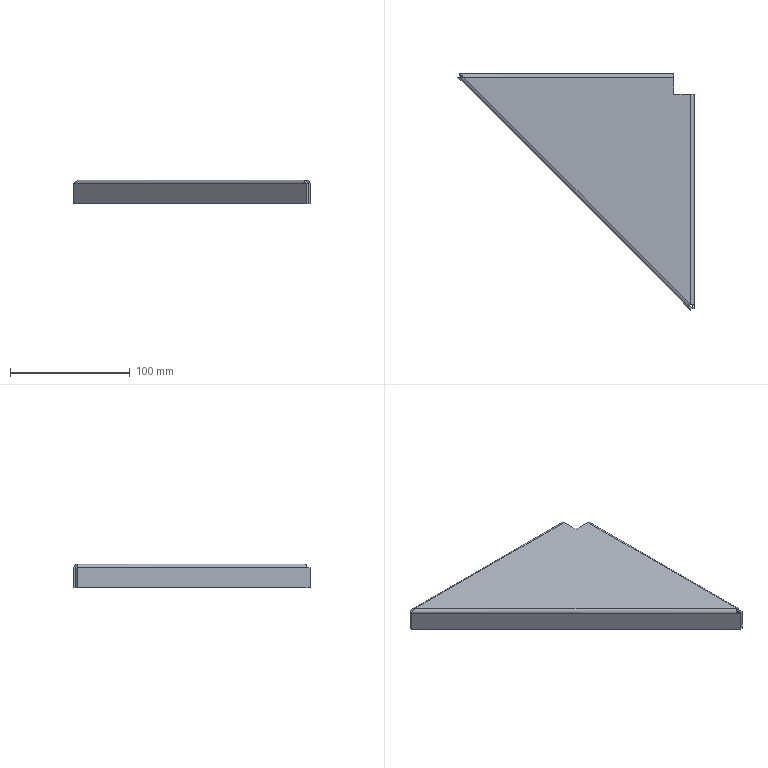Part | NX | features solid 2 | 1 solid | 45 faces | box 197.436 x 197.436 x 20 mm | volume 45854 mm3 | cylinder 22 | plane 21 | spline 2 | commonest cylinder face diameters 6 x19 3 x3
STEP:
#1=CARTESIAN_POINT('',(1090.,488.,1292.));
#2=VERTEX_POINT('',#1);
#3=CARTESIAN_POINT('',(1090.,488.,1275.));
#4=VERTEX_POINT('',#3);
#5=CARTESIAN_POINT('',(1090.,488.,1295.));
#6=DIRECTION('',(0.,0.,-1.));
#7=VECTOR('',#6,1000.);
#8=LINE('',#5,#7);
#9=EDGE_CURVE('',#2,#4,#8,.T.);
#10=ORIENTED_EDGE('',*,*,#9,.T.);
#11=CARTESIAN_POINT('',(1088.5,488.,1275.));
#12=VERTEX_POINT('',#11);
#13=CARTESIAN_POINT('',(1090.,488.,1275.));
#14=DIRECTION('',(1.,0.,0.));
#15=VECTOR('',#14,1000.);
#16=LINE('',#13,#15);
#17=EDGE_CURVE('',#12,#4,#16,.T.);
#18=ORIENTED_EDGE('',*,*,#17,.F.);
#19=CARTESIAN_POINT('',(1088.5,488.,1292.));
#20=VERTEX_POINT('',#19);
#21=CARTESIAN_POINT('',(1088.5,488.,1295.));
#22=DIRECTION('',(0.,0.,-1.));
#23=VECTOR('',#22,1000.);
#24=LINE('',#21,#23);
#25=EDGE_CURVE('',#20,#12,#24,.T.);
#26=ORIENTED_EDGE('',*,*,#25,.F.);
#27=CARTESIAN_POINT('',(1087.,488.,1293.5));
#28=VERTEX_POINT('',#27);
#29=CARTESIAN_POINT('',(1087.,488.,1292.));
#30=DIRECTION('',(0.,1.,0.));
#31=DIRECTION('',(0.,0.,1.));
#32=AXIS2_PLACEMENT_3D('',#29,#30,#31);
#33=CIRCLE('',#32,1.5);
#34=EDGE_CURVE('',#28,#20,#33,.T.);
#35=ORIENTED_EDGE('',*,*,#34,.F.);
#36=CARTESIAN_POINT('',(1073.,488.,1293.5));
#37=VERTEX_POINT('',#36);
#38=CARTESIAN_POINT('',(990.,488.,1293.5));
#39=DIRECTION('',(1.,0.,0.));
#40=VECTOR('',#39,1000.);
#41=LINE('',#38,#40);
#42=EDGE_CURVE('',#37,#28,#41,.T.);
#43=ORIENTED_EDGE('',*,*,#42,.F.);
#44=CARTESIAN_POINT('',(1073.,488.,1295.));
#45=VERTEX_POINT('',#44);
#46=CARTESIAN_POINT('',(1073.,488.,1295.));
#47=DIRECTION('',(0.,0.,1.));
#48=VECTOR('',#47,1000.);
#49=LINE('',#46,#48);
#50=EDGE_CURVE('',#37,#45,#49,.T.);
#51=ORIENTED_EDGE('',*,*,#50,.T.);
#52=CARTESIAN_POINT('',(1087.,488.,1295.));
#53=VERTEX_POINT('',#52);
#54=CARTESIAN_POINT('',(990.,488.,1295.));
#55=DIRECTION('',(1.,0.,0.));
#56=VECTOR('',#55,1000.);
#57=LINE('',#54,#56);
#58=EDGE_CURVE('',#45,#53,#57,.T.);
#59=ORIENTED_EDGE('',*,*,#58,.T.);
#60=CARTESIAN_POINT('',(1087.,488.,1292.));
#61=DIRECTION('',(0.,1.,0.));
#62=DIRECTION('',(0.,0.,1.));
#63=AXIS2_PLACEMENT_3D('',#60,#61,#62);
#64=CIRCLE('',#63,3.);
#65=EDGE_CURVE('',#53,#2,#64,.T.);
#66=ORIENTED_EDGE('',*,*,#65,.T.);
#67=EDGE_LOOP('',(#10,#18,#26,#35,#43,#51,#59,#66));
#68=FACE_BOUND('',#67,.T.);
#69=CARTESIAN_POINT('',(1090.,488.,1295.));
#70=DIRECTION('',(0.,-1.,0.));
#71=DIRECTION('',(-1.,0.,0.));
#72=AXIS2_PLACEMENT_3D('',#69,#70,#71);
#73=PLANE('',#72);
#74=ADVANCED_FACE('',(#68),#73,.F.);
#75=CARTESIAN_POINT('',(1073.,502.,1295.));
#76=VERTEX_POINT('',#75);
#77=CARTESIAN_POINT('',(1073.,405.,1295.));
#78=DIRECTION('',(0.,-1.,0.));
#79=VECTOR('',#78,1000.);
#80=LINE('',#77,#79);
#81=EDGE_CURVE('',#76,#45,#80,.T.);
#82=ORIENTED_EDGE('',*,*,#81,.T.);
#83=ORIENTED_EDGE('',*,*,#50,.F.);
#84=CARTESIAN_POINT('',(1073.,502.,1293.5));
#85=VERTEX_POINT('',#84);
#86=CARTESIAN_POINT('',(1073.,405.,1293.5));
#87=DIRECTION('',(0.,-1.,0.));
#88=VECTOR('',#87,1000.);
#89=LINE('',#86,#88);
#90=EDGE_CURVE('',#85,#37,#89,.T.);
#91=ORIENTED_EDGE('',*,*,#90,.F.);
#92=CARTESIAN_POINT('',(1073.,503.5,1292.));
#93=VERTEX_POINT('',#92);
#94=CARTESIAN_POINT('',(1073.,502.,1292.));
#95=DIRECTION('',(1.,0.,0.));
#96=DIRECTION('',(0.,1.,0.));
#97=AXIS2_PLACEMENT_3D('',#94,#95,#96);
#98=CIRCLE('',#97,1.5);
#99=EDGE_CURVE('',#93,#85,#98,.T.);
#100=ORIENTED_EDGE('',*,*,#99,.F.);
#101=CARTESIAN_POINT('',(1073.,503.5,1275.));
#102=VERTEX_POINT('',#101);
#103=CARTESIAN_POINT('',(1073.,503.5,1295.));
#104=DIRECTION('',(0.,0.,1.));
#105=VECTOR('',#104,1000.);
#106=LINE('',#103,#105);
#107=EDGE_CURVE('',#102,#93,#106,.T.);
#108=ORIENTED_EDGE('',*,*,#107,.F.);
#109=CARTESIAN_POINT('',(1073.,505.,1275.));
#110=VERTEX_POINT('',#109);
#111=CARTESIAN_POINT('',(1073.,505.,1275.));
#112=DIRECTION('',(0.,1.,0.));
#113=VECTOR('',#112,1000.);
#114=LINE('',#111,#113);
#115=EDGE_CURVE('',#102,#110,#114,.T.);
#116=ORIENTED_EDGE('',*,*,#115,.T.);
#117=CARTESIAN_POINT('',(1073.,505.,1292.));
#118=VERTEX_POINT('',#117);
#119=CARTESIAN_POINT('',(1073.,505.,1295.));
#120=DIRECTION('',(0.,0.,1.));
#121=VECTOR('',#120,1000.);
#122=LINE('',#119,#121);
#123=EDGE_CURVE('',#110,#118,#122,.T.);
#124=ORIENTED_EDGE('',*,*,#123,.T.);
#125=CARTESIAN_POINT('',(1073.,502.,1292.));
#126=DIRECTION('',(1.,0.,0.));
#127=DIRECTION('',(0.,0.,-1.));
#128=AXIS2_PLACEMENT_3D('',#125,#126,#127);
#129=CIRCLE('',#128,3.);
#130=EDGE_CURVE('',#118,#76,#129,.T.);
#131=ORIENTED_EDGE('',*,*,#130,.T.);
#132=EDGE_LOOP('',(#82,#83,#91,#100,#108,#116,#124,#131));
#133=FACE_BOUND('',#132,.T.);
#134=CARTESIAN_POINT('',(1073.,405.,1295.));
#135=DIRECTION('',(-1.,0.,0.));
#136=DIRECTION('',(0.,1.,0.));
#137=AXIS2_PLACEMENT_3D('',#134,#135,#136);
#138=PLANE('',#137);
#139=ADVANCED_FACE('',(#133),#138,.F.);
#140=CARTESIAN_POINT('',(1090.,480.,1282.));
#141=VERTEX_POINT('',#140);
#142=CARTESIAN_POINT('',(1088.5,480.,1282.));
#143=VERTEX_POINT('',#142);
#144=CARTESIAN_POINT('',(810.061,480.,1282.));
#145=DIRECTION('',(1.,0.,0.));
#146=VECTOR('',#145,1000.);
#147=LINE('',#144,#146);
#148=EDGE_CURVE('',#141,#143,#147,.F.);
#149=ORIENTED_EDGE('',*,*,#148,.T.);
#150=CARTESIAN_POINT('',(1088.5,480.,1288.));
#151=VERTEX_POINT('',#150);
#152=CARTESIAN_POINT('',(1088.5,480.,1285.));
#153=DIRECTION('',(1.,0.,0.));
#154=DIRECTION('',(0.,0.,1.));
#155=AXIS2_PLACEMENT_3D('',#152,#153,#154);
#156=CIRCLE('',#155,3.);
#157=EDGE_CURVE('',#151,#143,#156,.T.);
#158=ORIENTED_EDGE('',*,*,#157,.F.);
#159=CARTESIAN_POINT('',(1090.,480.,1288.));
#160=VERTEX_POINT('',#159);
#161=CARTESIAN_POINT('',(810.061,480.,1288.));
#162=DIRECTION('',(1.,0.,0.));
#163=VECTOR('',#162,1000.);
#164=LINE('',#161,#163);
#165=EDGE_CURVE('',#151,#160,#164,.T.);
#166=ORIENTED_EDGE('',*,*,#165,.T.);
#167=CARTESIAN_POINT('',(1090.,480.,1285.));
#168=DIRECTION('',(1.,0.,0.));
#169=DIRECTION('',(0.,1.,0.));
#170=AXIS2_PLACEMENT_3D('',#167,#168,#169);
#171=CIRCLE('',#170,3.);
#172=EDGE_CURVE('',#160,#141,#171,.T.);
#173=ORIENTED_EDGE('',*,*,#172,.T.);
#174=EDGE_LOOP('',(#149,#158,#166,#173));
#175=FACE_BOUND('',#174,.T.);
#176=CARTESIAN_POINT('',(810.061,480.,1285.));
#177=DIRECTION('',(1.,0.,0.));
#178=DIRECTION('',(0.,0.,1.));
#179=AXIS2_PLACEMENT_3D('',#176,#177,#178);
#180=CYLINDRICAL_SURFACE('',#179,3.);
#181=ADVANCED_FACE('',(#175),#180,.F.);
#182=CARTESIAN_POINT('',(1088.5,430.,1282.));
#183=VERTEX_POINT('',#182);
#184=CARTESIAN_POINT('',(1090.,430.,1282.));
#185=VERTEX_POINT('',#184);
#186=CARTESIAN_POINT('',(810.061,430.,1282.));
#187=DIRECTION('',(1.,0.,0.));
#188=VECTOR('',#187,1000.);
#189=LINE('',#186,#188);
#190=EDGE_CURVE('',#183,#185,#189,.T.);
#191=ORIENTED_EDGE('',*,*,#190,.F.);
#192=CARTESIAN_POINT('',(1088.5,430.,1288.));
#193=VERTEX_POINT('',#192);
#194=CARTESIAN_POINT('',(1088.5,430.,1285.));
#195=DIRECTION('',(1.,0.,0.));
#196=DIRECTION('',(0.,0.,1.));
#197=AXIS2_PLACEMENT_3D('',#194,#195,#196);
#198=CIRCLE('',#197,3.);
#199=EDGE_CURVE('',#193,#183,#198,.T.);
#200=ORIENTED_EDGE('',*,*,#199,.F.);
#201=CARTESIAN_POINT('',(1090.,430.,1288.));
#202=VERTEX_POINT('',#201);
#203=CARTESIAN_POINT('',(810.061,430.,1288.));
#204=DIRECTION('',(1.,0.,0.));
#205=VECTOR('',#204,1000.);
#206=LINE('',#203,#205);
#207=EDGE_CURVE('',#202,#193,#206,.F.);
#208=ORIENTED_EDGE('',*,*,#207,.F.);
#209=CARTESIAN_POINT('',(1090.,430.,1285.));
#210=DIRECTION('',(1.,0.,0.));
#211=DIRECTION('',(0.,1.,0.));
#212=AXIS2_PLACEMENT_3D('',#209,#210,#211);
#213=CIRCLE('',#212,3.);
#214=EDGE_CURVE('',#202,#185,#213,.T.);
#215=ORIENTED_EDGE('',*,*,#214,.T.);
#216=EDGE_LOOP('',(#191,#200,#208,#215));
#217=FACE_BOUND('',#216,.T.);
#218=CARTESIAN_POINT('',(810.061,430.,1285.));
#219=DIRECTION('',(1.,0.,0.));
#220=DIRECTION('',(0.,0.,1.));
#221=AXIS2_PLACEMENT_3D('',#218,#219,#220);
#222=CYLINDRICAL_SURFACE('',#221,3.);
#223=ADVANCED_FACE('',(#217),#222,.F.);
#224=CARTESIAN_POINT('',(1090.,380.,1282.));
#225=VERTEX_POINT('',#224);
#226=CARTESIAN_POINT('',(1088.5,380.,1282.));
#227=VERTEX_POINT('',#226);
#228=CARTESIAN_POINT('',(810.061,380.,1282.));
#229=DIRECTION('',(1.,0.,0.));
#230=VECTOR('',#229,1000.);
#231=LINE('',#228,#230);
#232=EDGE_CURVE('',#225,#227,#231,.F.);
#233=ORIENTED_EDGE('',*,*,#232,.T.);
#234=CARTESIAN_POINT('',(1088.5,380.,1288.));
#235=VERTEX_POINT('',#234);
#236=CARTESIAN_POINT('',(1088.5,380.,1285.));
#237=DIRECTION('',(1.,0.,0.));
#238=DIRECTION('',(0.,0.,1.));
#239=AXIS2_PLACEMENT_3D('',#236,#237,#238);
#240=CIRCLE('',#239,3.);
#241=EDGE_CURVE('',#235,#227,#240,.T.);
#242=ORIENTED_EDGE('',*,*,#241,.F.);
#243=CARTESIAN_POINT('',(1090.,380.,1288.));
#244=VERTEX_POINT('',#243);
#245=CARTESIAN_POINT('',(810.061,380.,1288.));
#246=DIRECTION('',(1.,0.,0.));
#247=VECTOR('',#246,1000.);
#248=LINE('',#245,#247);
#249=EDGE_CURVE('',#235,#244,#248,.T.);
#250=ORIENTED_EDGE('',*,*,#249,.T.);
#251=CARTESIAN_POINT('',(1090.,380.,1285.));
#252=DIRECTION('',(1.,0.,0.));
#253=DIRECTION('',(0.,1.,0.));
#254=AXIS2_PLACEMENT_3D('',#251,#252,#253);
#255=CIRCLE('',#254,3.);
#256=EDGE_CURVE('',#244,#225,#255,.T.);
#257=ORIENTED_EDGE('',*,*,#256,.T.);
#258=EDGE_LOOP('',(#233,#242,#250,#257));
#259=FACE_BOUND('',#258,.T.);
#260=CARTESIAN_POINT('',(810.061,380.,1285.));
#261=DIRECTION('',(1.,0.,0.));
#262=DIRECTION('',(0.,0.,1.));
#263=AXIS2_PLACEMENT_3D('',#260,#261,#262);
#264=CYLINDRICAL_SURFACE('',#263,3.);
#265=ADVANCED_FACE('',(#259),#264,.F.);
#266=CARTESIAN_POINT('',(1088.5,330.,1282.));
#267=VERTEX_POINT('',#266);
#268=CARTESIAN_POINT('',(1090.,330.,1282.));
#269=VERTEX_POINT('',#268);
#270=CARTESIAN_POINT('',(810.061,330.,1282.));
#271=DIRECTION('',(1.,0.,0.));
#272=VECTOR('',#271,1000.);
#273=LINE('',#270,#272);
#274=EDGE_CURVE('',#267,#269,#273,.T.);
#275=ORIENTED_EDGE('',*,*,#274,.F.);
#276=CARTESIAN_POINT('',(1088.5,330.,1288.));
#277=VERTEX_POINT('',#276);
#278=CARTESIAN_POINT('',(1088.5,330.,1285.));
#279=DIRECTION('',(1.,0.,0.));
#280=DIRECTION('',(0.,0.,1.));
#281=AXIS2_PLACEMENT_3D('',#278,#279,#280);
#282=CIRCLE('',#281,3.);
#283=EDGE_CURVE('',#277,#267,#282,.T.);
#284=ORIENTED_EDGE('',*,*,#283,.F.);
#285=CARTESIAN_POINT('',(1090.,330.,1288.));
#286=VERTEX_POINT('',#285);
#287=CARTESIAN_POINT('',(810.061,330.,1288.));
#288=DIRECTION('',(1.,0.,0.));
#289=VECTOR('',#288,1000.);
#290=LINE('',#287,#289);
#291=EDGE_CURVE('',#286,#277,#290,.F.);
#292=ORIENTED_EDGE('',*,*,#291,.F.);
#293=CARTESIAN_POINT('',(1090.,330.,1285.));
#294=DIRECTION('',(1.,0.,0.));
#295=DIRECTION('',(0.,1.,0.));
#296=AXIS2_PLACEMENT_3D('',#293,#294,#295);
#297=CIRCLE('',#296,3.);
#298=EDGE_CURVE('',#286,#269,#297,.T.);
#299=ORIENTED_EDGE('',*,*,#298,.T.);
#300=EDGE_LOOP('',(#275,#284,#292,#299));
#301=FACE_BOUND('',#300,.T.);
#302=CARTESIAN_POINT('',(810.061,330.,1285.));
#303=DIRECTION('',(1.,0.,0.));
#304=DIRECTION('',(0.,0.,1.));
#305=AXIS2_PLACEMENT_3D('',#302,#303,#304);
#306=CYLINDRICAL_SURFACE('',#305,3.);
#307=ADVANCED_FACE('',(#301),#306,.F.);
#308=CARTESIAN_POINT('',(915.,505.,1288.));
#309=VERTEX_POINT('',#308);
#310=CARTESIAN_POINT('',(915.,503.5,1288.));
#311=VERTEX_POINT('',#310);
#312=CARTESIAN_POINT('',(915.,225.061,1288.));
#313=DIRECTION('',(0.,1.,0.));
#314=VECTOR('',#313,1000.);
#315=LINE('',#312,#314);
#316=EDGE_CURVE('',#309,#311,#315,.F.);
#317=ORIENTED_EDGE('',*,*,#316,.T.);
#318=CARTESIAN_POINT('',(915.,503.5,1282.));
#319=VERTEX_POINT('',#318);
#320=CARTESIAN_POINT('',(915.,503.5,1285.));
#321=DIRECTION('',(0.,1.,0.));
#322=DIRECTION('',(0.,0.,-1.));
#323=AXIS2_PLACEMENT_3D('',#320,#321,#322);
#324=CIRCLE('',#323,3.);
#325=EDGE_CURVE('',#319,#311,#324,.T.);
#326=ORIENTED_EDGE('',*,*,#325,.F.);
#327=CARTESIAN_POINT('',(915.,505.,1282.));
#328=VERTEX_POINT('',#327);
#329=CARTESIAN_POINT('',(915.,225.061,1282.));
#330=DIRECTION('',(0.,1.,0.));
#331=VECTOR('',#330,1000.);
#332=LINE('',#329,#331);
#333=EDGE_CURVE('',#319,#328,#332,.T.);
#334=ORIENTED_EDGE('',*,*,#333,.T.);
#335=CARTESIAN_POINT('',(915.,505.,1285.));
#336=DIRECTION('',(0.,1.,0.));
#337=DIRECTION('',(-1.,0.,0.));
#338=AXIS2_PLACEMENT_3D('',#335,#336,#337);
#339=CIRCLE('',#338,3.);
#340=EDGE_CURVE('',#328,#309,#339,.T.);
#341=ORIENTED_EDGE('',*,*,#340,.T.);
#342=EDGE_LOOP('',(#317,#326,#334,#341));
#343=FACE_BOUND('',#342,.T.);
#344=CARTESIAN_POINT('',(915.,225.061,1285.));
#345=DIRECTION('',(0.,1.,0.));
#346=DIRECTION('',(0.,0.,-1.));
#347=AXIS2_PLACEMENT_3D('',#344,#345,#346);
#348=CYLINDRICAL_SURFACE('',#347,3.);
#349=ADVANCED_FACE('',(#343),#348,.F.);
#350=CARTESIAN_POINT('',(965.,503.5,1288.));
#351=VERTEX_POINT('',#350);
#352=CARTESIAN_POINT('',(965.,505.,1288.));
#353=VERTEX_POINT('',#352);
#354=CARTESIAN_POINT('',(965.,225.061,1288.));
#355=DIRECTION('',(0.,1.,0.));
#356=VECTOR('',#355,1000.);
#357=LINE('',#354,#356);
#358=EDGE_CURVE('',#351,#353,#357,.T.);
#359=ORIENTED_EDGE('',*,*,#358,.F.);
#360=CARTESIAN_POINT('',(965.,503.5,1282.));
#361=VERTEX_POINT('',#360);
#362=CARTESIAN_POINT('',(965.,503.5,1285.));
#363=DIRECTION('',(0.,1.,0.));
#364=DIRECTION('',(0.,0.,-1.));
#365=AXIS2_PLACEMENT_3D('',#362,#363,#364);
#366=CIRCLE('',#365,3.);
#367=EDGE_CURVE('',#361,#351,#366,.T.);
#368=ORIENTED_EDGE('',*,*,#367,.F.);
#369=CARTESIAN_POINT('',(965.,505.,1282.));
#370=VERTEX_POINT('',#369);
#371=CARTESIAN_POINT('',(965.,225.061,1282.));
#372=DIRECTION('',(0.,1.,0.));
#373=VECTOR('',#372,1000.);
#374=LINE('',#371,#373);
#375=EDGE_CURVE('',#370,#361,#374,.F.);
#376=ORIENTED_EDGE('',*,*,#375,.F.);
#377=CARTESIAN_POINT('',(965.,505.,1285.));
#378=DIRECTION('',(0.,1.,0.));
#379=DIRECTION('',(-1.,0.,0.));
#380=AXIS2_PLACEMENT_3D('',#377,#378,#379);
#381=CIRCLE('',#380,3.);
#382=EDGE_CURVE('',#370,#353,#381,.T.);
#383=ORIENTED_EDGE('',*,*,#382,.T.);
#384=EDGE_LOOP('',(#359,#368,#376,#383));
#385=FACE_BOUND('',#384,.T.);
#386=CARTESIAN_POINT('',(965.,225.061,1285.));
#387=DIRECTION('',(0.,1.,0.));
#388=DIRECTION('',(0.,0.,-1.));
#389=AXIS2_PLACEMENT_3D('',#386,#387,#388);
#390=CYLINDRICAL_SURFACE('',#389,3.);
#391=ADVANCED_FACE('',(#385),#390,.F.);
#392=CARTESIAN_POINT('',(1015.,505.,1288.));
#393=VERTEX_POINT('',#392);
#394=CARTESIAN_POINT('',(1015.,503.5,1288.));
#395=VERTEX_POINT('',#394);
#396=CARTESIAN_POINT('',(1015.,225.061,1288.));
#397=DIRECTION('',(0.,1.,0.));
#398=VECTOR('',#397,1000.);
#399=LINE('',#396,#398);
#400=EDGE_CURVE('',#393,#395,#399,.F.);
#401=ORIENTED_EDGE('',*,*,#400,.T.);
#402=CARTESIAN_POINT('',(1015.,503.5,1282.));
#403=VERTEX_POINT('',#402);
#404=CARTESIAN_POINT('',(1015.,503.5,1285.));
#405=DIRECTION('',(0.,1.,0.));
#406=DIRECTION('',(0.,0.,-1.));
#407=AXIS2_PLACEMENT_3D('',#404,#405,#406);
#408=CIRCLE('',#407,3.);
#409=EDGE_CURVE('',#403,#395,#408,.T.);
#410=ORIENTED_EDGE('',*,*,#409,.F.);
#411=CARTESIAN_POINT('',(1015.,505.,1282.));
#412=VERTEX_POINT('',#411);
#413=CARTESIAN_POINT('',(1015.,225.061,1282.));
#414=DIRECTION('',(0.,1.,0.));
#415=VECTOR('',#414,1000.);
#416=LINE('',#413,#415);
#417=EDGE_CURVE('',#403,#412,#416,.T.);
#418=ORIENTED_EDGE('',*,*,#417,.T.);
#419=CARTESIAN_POINT('',(1015.,505.,1285.));
#420=DIRECTION('',(0.,1.,0.));
#421=DIRECTION('',(-1.,0.,0.));
#422=AXIS2_PLACEMENT_3D('',#419,#420,#421);
#423=CIRCLE('',#422,3.);
#424=EDGE_CURVE('',#412,#393,#423,.T.);
#425=ORIENTED_EDGE('',*,*,#424,.T.);
#426=EDGE_LOOP('',(#401,#410,#418,#425));
#427=FACE_BOUND('',#426,.T.);
#428=CARTESIAN_POINT('',(1015.,225.061,1285.));
#429=DIRECTION('',(0.,1.,0.));
#430=DIRECTION('',(0.,0.,-1.));
#431=AXIS2_PLACEMENT_3D('',#428,#429,#430);
#432=CYLINDRICAL_SURFACE('',#431,3.);
#433=ADVANCED_FACE('',(#427),#432,.F.);
#434=CARTESIAN_POINT('',(1065.,503.5,1288.));
#435=VERTEX_POINT('',#434);
#436=CARTESIAN_POINT('',(1065.,505.,1288.));
#437=VERTEX_POINT('',#436);
#438=CARTESIAN_POINT('',(1065.,225.061,1288.));
#439=DIRECTION('',(0.,1.,0.));
#440=VECTOR('',#439,1000.);
#441=LINE('',#438,#440);
#442=EDGE_CURVE('',#435,#437,#441,.T.);
#443=ORIENTED_EDGE('',*,*,#442,.F.);
#444=CARTESIAN_POINT('',(1065.,503.5,1282.));
#445=VERTEX_POINT('',#444);
#446=CARTESIAN_POINT('',(1065.,503.5,1285.));
#447=DIRECTION('',(0.,1.,0.));
#448=DIRECTION('',(0.,0.,-1.));
#449=AXIS2_PLACEMENT_3D('',#446,#447,#448);
#450=CIRCLE('',#449,3.);
#451=EDGE_CURVE('',#445,#435,#450,.T.);
#452=ORIENTED_EDGE('',*,*,#451,.F.);
#453=CARTESIAN_POINT('',(1065.,505.,1282.));
#454=VERTEX_POINT('',#453);
#455=CARTESIAN_POINT('',(1065.,225.061,1282.));
#456=DIRECTION('',(0.,1.,0.));
#457=VECTOR('',#456,1000.);
#458=LINE('',#455,#457);
#459=EDGE_CURVE('',#454,#445,#458,.F.);
#460=ORIENTED_EDGE('',*,*,#459,.F.);
#461=CARTESIAN_POINT('',(1065.,505.,1285.));
#462=DIRECTION('',(0.,1.,0.));
#463=DIRECTION('',(-1.,0.,0.));
#464=AXIS2_PLACEMENT_3D('',#461,#462,#463);
#465=CIRCLE('',#464,3.);
#466=EDGE_CURVE('',#454,#437,#465,.T.);
#467=ORIENTED_EDGE('',*,*,#466,.T.);
#468=EDGE_LOOP('',(#443,#452,#460,#467));
#469=FACE_BOUND('',#468,.T.);
#470=CARTESIAN_POINT('',(1065.,225.061,1285.));
#471=DIRECTION('',(0.,1.,0.));
#472=DIRECTION('',(0.,0.,-1.));
#473=AXIS2_PLACEMENT_3D('',#470,#471,#472);
#474=CYLINDRICAL_SURFACE('',#473,3.);
#475=ADVANCED_FACE('',(#469),#474,.F.);
#476=ORIENTED_EDGE('',*,*,#451,.T.);
#477=CARTESIAN_POINT('',(1065.,503.5,1285.));
#478=DIRECTION('',(0.,1.,0.));
#479=DIRECTION('',(0.,0.,-1.));
#480=AXIS2_PLACEMENT_3D('',#477,#478,#479);
#481=CIRCLE('',#480,3.);
#482=EDGE_CURVE('',#435,#445,#481,.T.);
#483=ORIENTED_EDGE('',*,*,#482,.T.);
#484=EDGE_LOOP('',(#476,#483));
#485=FACE_BOUND('',#484,.T.);
#486=ORIENTED_EDGE('',*,*,#409,.T.);
#487=CARTESIAN_POINT('',(1015.,503.5,1285.));
#488=DIRECTION('',(0.,1.,0.));
#489=DIRECTION('',(0.,0.,-1.));
#490=AXIS2_PLACEMENT_3D('',#487,#488,#489);
#491=CIRCLE('',#490,3.);
#492=EDGE_CURVE('',#395,#403,#491,.T.);
#493=ORIENTED_EDGE('',*,*,#492,.T.);
#494=EDGE_LOOP('',(#486,#493));
#495=FACE_BOUND('',#494,.T.);
#496=ORIENTED_EDGE('',*,*,#367,.T.);
#497=CARTESIAN_POINT('',(965.,503.5,1285.));
#498=DIRECTION('',(0.,1.,0.));
#499=DIRECTION('',(0.,0.,-1.));
#500=AXIS2_PLACEMENT_3D('',#497,#498,#499);
#501=CIRCLE('',#500,3.);
#502=EDGE_CURVE('',#351,#361,#501,.T.);
#503=ORIENTED_EDGE('',*,*,#502,.T.);
#504=EDGE_LOOP('',(#496,#503));
#505=FACE_BOUND('',#504,.T.);
#506=ORIENTED_EDGE('',*,*,#325,.T.);
#507=CARTESIAN_POINT('',(915.,503.5,1285.));
#508=DIRECTION('',(0.,1.,0.));
#509=DIRECTION('',(0.,0.,-1.));
#510=AXIS2_PLACEMENT_3D('',#507,#508,#509);
#511=CIRCLE('',#510,3.);
#512=EDGE_CURVE('',#311,#319,#511,.T.);
#513=ORIENTED_EDGE('',*,*,#512,.T.);
#514=EDGE_LOOP('',(#506,#513));
#515=FACE_BOUND('',#514,.T.);
#516=CARTESIAN_POINT('',(893.627,503.5,1275.));
#517=VERTEX_POINT('',#516);
#518=CARTESIAN_POINT('',(1667.136,503.5,1275.));
#519=DIRECTION('',(-1.,0.,0.));
#520=VECTOR('',#519,1000.);
#521=LINE('',#518,#520);
#522=EDGE_CURVE('',#102,#517,#521,.T.);
#523=ORIENTED_EDGE('',*,*,#522,.F.);
#524=ORIENTED_EDGE('',*,*,#107,.T.);
#525=CARTESIAN_POINT('',(893.627,503.5,1292.));
#526=VERTEX_POINT('',#525);
#527=CARTESIAN_POINT('',(1667.136,503.5,1292.));
#528=DIRECTION('',(-1.,0.,0.));
#529=VECTOR('',#528,1000.);
#530=LINE('',#527,#529);
#531=EDGE_CURVE('',#93,#526,#530,.T.);
#532=ORIENTED_EDGE('',*,*,#531,.T.);
#533=CARTESIAN_POINT('',(893.627,503.5,1295.));
#534=DIRECTION('',(0.,0.,-1.));
#535=VECTOR('',#534,1000.);
#536=LINE('',#533,#535);
#537=EDGE_CURVE('',#526,#517,#536,.T.);
#538=ORIENTED_EDGE('',*,*,#537,.T.);
#539=EDGE_LOOP('',(#523,#524,#532,#538));
#540=FACE_BOUND('',#539,.T.);
#541=CARTESIAN_POINT('',(1667.136,503.5,1295.));
#542=DIRECTION('',(0.,1.,0.));
#543=DIRECTION('',(1.,0.,0.));
#544=AXIS2_PLACEMENT_3D('',#541,#542,#543);
#545=PLANE('',#544);
#546=ADVANCED_FACE('',(#485,#495,#505,#515,#540),#545,.F.);
#547=ORIENTED_EDGE('',*,*,#466,.F.);
#548=CARTESIAN_POINT('',(1065.,505.,1285.));
#549=DIRECTION('',(0.,1.,0.));
#550=DIRECTION('',(-1.,0.,0.));
#551=AXIS2_PLACEMENT_3D('',#548,#549,#550);
#552=CIRCLE('',#551,3.);
#553=EDGE_CURVE('',#437,#454,#552,.T.);
#554=ORIENTED_EDGE('',*,*,#553,.F.);
#555=EDGE_LOOP('',(#547,#554));
#556=FACE_BOUND('',#555,.T.);
#557=ORIENTED_EDGE('',*,*,#424,.F.);
#558=CARTESIAN_POINT('',(1015.,505.,1285.));
#559=DIRECTION('',(0.,1.,0.));
#560=DIRECTION('',(-1.,0.,0.));
#561=AXIS2_PLACEMENT_3D('',#558,#559,#560);
#562=CIRCLE('',#561,3.);
#563=EDGE_CURVE('',#393,#412,#562,.T.);
#564=ORIENTED_EDGE('',*,*,#563,.F.);
#565=EDGE_LOOP('',(#557,#564));
#566=FACE_BOUND('',#565,.T.);
#567=ORIENTED_EDGE('',*,*,#382,.F.);
#568=CARTESIAN_POINT('',(965.,505.,1285.));
#569=DIRECTION('',(0.,1.,0.));
#570=DIRECTION('',(-1.,0.,0.));
#571=AXIS2_PLACEMENT_3D('',#568,#569,#570);
#572=CIRCLE('',#571,3.);
#573=EDGE_CURVE('',#353,#370,#572,.T.);
#574=ORIENTED_EDGE('',*,*,#573,.F.);
#575=EDGE_LOOP('',(#567,#574));
#576=FACE_BOUND('',#575,.T.);
#577=ORIENTED_EDGE('',*,*,#340,.F.);
#578=CARTESIAN_POINT('',(915.,505.,1285.));
#579=DIRECTION('',(0.,1.,0.));
#580=DIRECTION('',(-1.,0.,0.));
#581=AXIS2_PLACEMENT_3D('',#578,#579,#580);
#582=CIRCLE('',#581,3.);
#583=EDGE_CURVE('',#309,#328,#582,.T.);
#584=ORIENTED_EDGE('',*,*,#583,.F.);
#585=EDGE_LOOP('',(#577,#584));
#586=FACE_BOUND('',#585,.T.);
#587=ORIENTED_EDGE('',*,*,#123,.F.);
#588=CARTESIAN_POINT('',(893.627,505.,1275.));
#589=VERTEX_POINT('',#588);
#590=CARTESIAN_POINT('',(1667.136,505.,1275.));
#591=DIRECTION('',(-1.,0.,0.));
#592=VECTOR('',#591,1000.);
#593=LINE('',#590,#592);
#594=EDGE_CURVE('',#110,#589,#593,.T.);
#595=ORIENTED_EDGE('',*,*,#594,.T.);
#596=CARTESIAN_POINT('',(893.627,505.,1292.));
#597=VERTEX_POINT('',#596);
#598=CARTESIAN_POINT('',(893.627,505.,1295.));
#599=DIRECTION('',(0.,0.,-1.));
#600=VECTOR('',#599,1000.);
#601=LINE('',#598,#600);
#602=EDGE_CURVE('',#597,#589,#601,.T.);
#603=ORIENTED_EDGE('',*,*,#602,.F.);
#604=CARTESIAN_POINT('',(1667.136,505.,1292.));
#605=DIRECTION('',(-1.,0.,0.));
#606=VECTOR('',#605,1000.);
#607=LINE('',#604,#606);
#608=EDGE_CURVE('',#118,#597,#607,.T.);
#609=ORIENTED_EDGE('',*,*,#608,.F.);
#610=EDGE_LOOP('',(#587,#595,#603,#609));
#611=FACE_BOUND('',#610,.T.);
#612=CARTESIAN_POINT('',(1667.136,505.,1295.));
#613=DIRECTION('',(0.,1.,0.));
#614=DIRECTION('',(1.,0.,0.));
#615=AXIS2_PLACEMENT_3D('',#612,#613,#614);
#616=PLANE('',#615);
#617=ADVANCED_FACE('',(#556,#566,#576,#586,#611),#616,.T.);
#618=CARTESIAN_POINT('',(893.627,503.5,1275.));
#619=DIRECTION('',(0.,-1.,0.));
#620=VECTOR('',#619,1000.);
#621=LINE('',#618,#620);
#622=EDGE_CURVE('',#589,#517,#621,.T.);
#623=ORIENTED_EDGE('',*,*,#622,.T.);
#624=ORIENTED_EDGE('',*,*,#537,.F.);
#625=CARTESIAN_POINT('',(893.627,503.5,1292.));
#626=DIRECTION('',(0.,-1.,0.));
#627=VECTOR('',#626,1000.);
#628=LINE('',#625,#627);
#629=EDGE_CURVE('',#597,#526,#628,.T.);
#630=ORIENTED_EDGE('',*,*,#629,.F.);
#631=ORIENTED_EDGE('',*,*,#602,.T.);
#632=EDGE_LOOP('',(#623,#624,#630,#631));
#633=FACE_BOUND('',#632,.T.);
#634=CARTESIAN_POINT('',(893.627,503.5,1295.));
#635=DIRECTION('',(1.,0.,0.));
#636=DIRECTION('',(0.,0.,-1.));
#637=AXIS2_PLACEMENT_3D('',#634,#635,#636);
#638=PLANE('',#637);
#639=ADVANCED_FACE('',(#633),#638,.F.);
#640=ORIENTED_EDGE('',*,*,#115,.F.);
#641=ORIENTED_EDGE('',*,*,#522,.T.);
#642=ORIENTED_EDGE('',*,*,#622,.F.);
#643=ORIENTED_EDGE('',*,*,#594,.F.);
#644=EDGE_LOOP('',(#640,#641,#642,#643));
#645=FACE_BOUND('',#644,.T.);
#646=CARTESIAN_POINT('',(1667.136,505.,1275.));
#647=DIRECTION('',(0.,0.,-1.));
#648=DIRECTION('',(-1.,0.,0.));
#649=AXIS2_PLACEMENT_3D('',#646,#647,#648);
#650=PLANE('',#649);
#651=ADVANCED_FACE('',(#645),#650,.T.);
#652=ORIENTED_EDGE('',*,*,#629,.T.);
#653=CARTESIAN_POINT('',(897.243,502.,1293.5));
#654=VERTEX_POINT('',#653);
#655=CARTESIAN_POINT('',(897.243,502.,1293.5));
#656=CARTESIAN_POINT('',(896.037,502.785,1293.5));
#657=CARTESIAN_POINT('',(894.832,503.5,1292.785));
#658=CARTESIAN_POINT('',(893.627,503.5,1292.));
#659=B_SPLINE_CURVE_WITH_KNOTS('',3,(#655,#656,#657,#658),.UNSPECIFIED.,.F.,.F.,(4,4),(0.,1.),.UNSPECIFIED.);
#660=EDGE_CURVE('',#526,#654,#659,.F.);
#661=ORIENTED_EDGE('',*,*,#660,.T.);
#662=CARTESIAN_POINT('',(897.243,502.,1295.));
#663=VERTEX_POINT('',#662);
#664=CARTESIAN_POINT('',(897.243,502.,1295.));
#665=DIRECTION('',(0.,0.,1.));
#666=VECTOR('',#665,1000.);
#667=LINE('',#664,#666);
#668=EDGE_CURVE('',#654,#663,#667,.T.);
#669=ORIENTED_EDGE('',*,*,#668,.T.);
#670=CARTESIAN_POINT('',(893.627,505.,1292.));
#671=CARTESIAN_POINT('',(894.229,505.,1292.785));
#672=CARTESIAN_POINT('',(895.435,504.35,1294.35));
#673=CARTESIAN_POINT('',(896.64,502.785,1295.));
#674=CARTESIAN_POINT('',(897.243,502.,1295.));
#675=B_SPLINE_CURVE_WITH_KNOTS('',3,(#670,#671,#672,#673,#674),.UNSPECIFIED.,.F.,.F.,(4,1,4),(0.,0.5,1.),.UNSPECIFIED.);
#676=EDGE_CURVE('',#597,#663,#675,.T.);
#677=ORIENTED_EDGE('',*,*,#676,.F.);
#678=EDGE_LOOP('',(#652,#661,#669,#677));
#679=FACE_BOUND('',#678,.T.);
#680=CARTESIAN_POINT('',(893.627,505.,1292.));
#681=CARTESIAN_POINT('',(893.928,505.,1292.393));
#682=CARTESIAN_POINT('',(894.229,504.922,1292.785));
#683=CARTESIAN_POINT('',(894.832,504.621,1293.511));
#684=CARTESIAN_POINT('',(895.133,504.399,1293.844));
#685=CARTESIAN_POINT('',(895.736,503.844,1294.399));
#686=CARTESIAN_POINT('',(896.037,503.511,1294.621));
#687=CARTESIAN_POINT('',(896.64,502.785,1294.922));
#688=CARTESIAN_POINT('',(896.941,502.393,1295.));
#689=CARTESIAN_POINT('',(897.243,502.,1295.));
#690=CARTESIAN_POINT('',(893.627,503.5,1292.));
#691=CARTESIAN_POINT('',(893.928,503.5,1292.196));
#692=CARTESIAN_POINT('',(894.229,503.461,1292.393));
#693=CARTESIAN_POINT('',(894.832,503.311,1292.755));
#694=CARTESIAN_POINT('',(895.133,503.2,1292.922));
#695=CARTESIAN_POINT('',(895.736,502.922,1293.2));
#696=CARTESIAN_POINT('',(896.037,502.755,1293.311));
#697=CARTESIAN_POINT('',(896.64,502.393,1293.461));
#698=CARTESIAN_POINT('',(896.941,502.196,1293.5));
#699=CARTESIAN_POINT('',(897.243,502.,1293.5));
#700=(BOUNDED_SURFACE()B_SPLINE_SURFACE(1,3,((#680,#681,#682,#683,#684,#685,#686,#687,#688,#689),(#690,#691,#692,#693,#694,#695,#696,#697,#698,#699)),.RULED_SURF.,.F.,.F.,.F.)B_SPLINE_SURFACE_WITH_KNOTS((2,2),(4,2,2,2,4),(0.,1.),(0.,0.25,0.5,0.75,1.),.UNSPECIFIED.)GEOMETRIC_REPRESENTATION_ITEM()RATIONAL_B_SPLINE_SURFACE(((1.,1.,1.,1.,1.,1.,1.,1.,1.,1.),(1.,1.,1.,1.,1.,1.,1.,1.,1.,1.)))REPRESENTATION_ITEM('')SURFACE());
#701=ADVANCED_FACE('',(#679),#700,.T.);
#702=ORIENTED_EDGE('',*,*,#130,.F.);
#703=ORIENTED_EDGE('',*,*,#608,.T.);
#704=ORIENTED_EDGE('',*,*,#676,.T.);
#705=CARTESIAN_POINT('',(897.243,502.,1295.));
#706=DIRECTION('',(1.,0.,0.));
#707=VECTOR('',#706,1000.);
#708=LINE('',#705,#707);
#709=EDGE_CURVE('',#663,#76,#708,.T.);
#710=ORIENTED_EDGE('',*,*,#709,.T.);
#711=EDGE_LOOP('',(#702,#703,#704,#710));
#712=FACE_BOUND('',#711,.T.);
#713=CARTESIAN_POINT('',(1087.,502.,1292.));
#714=DIRECTION('',(1.,0.,0.));
#715=DIRECTION('',(0.,0.,-1.));
#716=AXIS2_PLACEMENT_3D('',#713,#714,#715);
#717=CYLINDRICAL_SURFACE('',#716,3.);
#718=ADVANCED_FACE('',(#712),#717,.T.);
#719=ORIENTED_EDGE('',*,*,#531,.F.);
#720=ORIENTED_EDGE('',*,*,#99,.T.);
#721=CARTESIAN_POINT('',(1087.,502.,1293.5));
#722=DIRECTION('',(1.,0.,0.));
#723=VECTOR('',#722,1000.);
#724=LINE('',#721,#723);
#725=EDGE_CURVE('',#654,#85,#724,.T.);
#726=ORIENTED_EDGE('',*,*,#725,.F.);
#727=ORIENTED_EDGE('',*,*,#660,.F.);
#728=EDGE_LOOP('',(#719,#720,#726,#727));
#729=FACE_BOUND('',#728,.T.);
#730=CARTESIAN_POINT('',(1087.,502.,1292.));
#731=DIRECTION('',(1.,0.,0.));
#732=DIRECTION('',(0.,0.,-1.));
#733=AXIS2_PLACEMENT_3D('',#730,#731,#732);
#734=CYLINDRICAL_SURFACE('',#733,1.5);
#735=ADVANCED_FACE('',(#729),#734,.F.);
#736=ORIENTED_EDGE('',*,*,#298,.F.);
#737=CARTESIAN_POINT('',(1090.,330.,1285.));
#738=DIRECTION('',(1.,0.,0.));
#739=DIRECTION('',(0.,1.,0.));
#740=AXIS2_PLACEMENT_3D('',#737,#738,#739);
#741=CIRCLE('',#740,3.);
#742=EDGE_CURVE('',#269,#286,#741,.T.);
#743=ORIENTED_EDGE('',*,*,#742,.F.);
#744=EDGE_LOOP('',(#736,#743));
#745=FACE_BOUND('',#744,.T.);
#746=ORIENTED_EDGE('',*,*,#256,.F.);
#747=CARTESIAN_POINT('',(1090.,380.,1285.));
#748=DIRECTION('',(1.,0.,0.));
#749=DIRECTION('',(0.,1.,0.));
#750=AXIS2_PLACEMENT_3D('',#747,#748,#749);
#751=CIRCLE('',#750,3.);
#752=EDGE_CURVE('',#225,#244,#751,.T.);
#753=ORIENTED_EDGE('',*,*,#752,.F.);
#754=EDGE_LOOP('',(#746,#753));
#755=FACE_BOUND('',#754,.T.);
#756=ORIENTED_EDGE('',*,*,#214,.F.);
#757=CARTESIAN_POINT('',(1090.,430.,1285.));
#758=DIRECTION('',(1.,0.,0.));
#759=DIRECTION('',(0.,1.,0.));
#760=AXIS2_PLACEMENT_3D('',#757,#758,#759);
#761=CIRCLE('',#760,3.);
#762=EDGE_CURVE('',#185,#202,#761,.T.);
#763=ORIENTED_EDGE('',*,*,#762,.F.);
#764=EDGE_LOOP('',(#756,#763));
#765=FACE_BOUND('',#764,.T.);
#766=ORIENTED_EDGE('',*,*,#172,.F.);
#767=CARTESIAN_POINT('',(1090.,480.,1285.));
#768=DIRECTION('',(1.,0.,0.));
#769=DIRECTION('',(0.,1.,0.));
#770=AXIS2_PLACEMENT_3D('',#767,#768,#769);
#771=CIRCLE('',#770,3.);
#772=EDGE_CURVE('',#141,#160,#771,.T.);
#773=ORIENTED_EDGE('',*,*,#772,.F.);
#774=EDGE_LOOP('',(#766,#773));
#775=FACE_BOUND('',#774,.T.);
#776=ORIENTED_EDGE('',*,*,#9,.F.);
#777=CARTESIAN_POINT('',(1090.,312.243,1292.));
#778=VERTEX_POINT('',#777);
#779=CARTESIAN_POINT('',(1090.,-273.529,1292.));
#780=DIRECTION('',(0.,1.,0.));
#781=VECTOR('',#780,1000.);
#782=LINE('',#779,#781);
#783=EDGE_CURVE('',#778,#2,#782,.T.);
#784=ORIENTED_EDGE('',*,*,#783,.F.);
#785=CARTESIAN_POINT('',(1090.,308.627,1292.));
#786=VERTEX_POINT('',#785);
#787=CARTESIAN_POINT('',(1090.,-273.529,1292.));
#788=DIRECTION('',(0.,1.,0.));
#789=VECTOR('',#788,1000.);
#790=LINE('',#787,#789);
#791=EDGE_CURVE('',#786,#778,#790,.T.);
#792=ORIENTED_EDGE('',*,*,#791,.F.);
#793=CARTESIAN_POINT('',(1090.,308.627,1275.));
#794=VERTEX_POINT('',#793);
#795=CARTESIAN_POINT('',(1090.,308.627,1295.));
#796=DIRECTION('',(0.,0.,1.));
#797=VECTOR('',#796,1000.);
#798=LINE('',#795,#797);
#799=EDGE_CURVE('',#794,#786,#798,.T.);
#800=ORIENTED_EDGE('',*,*,#799,.F.);
#801=CARTESIAN_POINT('',(1090.,-273.529,1275.));
#802=DIRECTION('',(0.,1.,0.));
#803=VECTOR('',#802,1000.);
#804=LINE('',#801,#803);
#805=EDGE_CURVE('',#794,#4,#804,.T.);
#806=ORIENTED_EDGE('',*,*,#805,.T.);
#807=EDGE_LOOP('',(#776,#784,#792,#800,#806));
#808=FACE_BOUND('',#807,.T.);
#809=CARTESIAN_POINT('',(1090.,-273.529,1295.));
#810=DIRECTION('',(1.,0.,0.));
#811=DIRECTION('',(0.,-1.,0.));
#812=AXIS2_PLACEMENT_3D('',#809,#810,#811);
#813=PLANE('',#812);
#814=ADVANCED_FACE('',(#745,#755,#765,#775,#808),#813,.T.);
#815=ORIENTED_EDGE('',*,*,#283,.T.);
#816=CARTESIAN_POINT('',(1088.5,330.,1285.));
#817=DIRECTION('',(1.,0.,0.));
#818=DIRECTION('',(0.,0.,1.));
#819=AXIS2_PLACEMENT_3D('',#816,#817,#818);
#820=CIRCLE('',#819,3.);
#821=EDGE_CURVE('',#267,#277,#820,.T.);
#822=ORIENTED_EDGE('',*,*,#821,.T.);
#823=EDGE_LOOP('',(#815,#822));
#824=FACE_BOUND('',#823,.T.);
#825=ORIENTED_EDGE('',*,*,#241,.T.);
#826=CARTESIAN_POINT('',(1088.5,380.,1285.));
#827=DIRECTION('',(1.,0.,0.));
#828=DIRECTION('',(0.,0.,1.));
#829=AXIS2_PLACEMENT_3D('',#826,#827,#828);
#830=CIRCLE('',#829,3.);
#831=EDGE_CURVE('',#227,#235,#830,.T.);
#832=ORIENTED_EDGE('',*,*,#831,.T.);
#833=EDGE_LOOP('',(#825,#832));
#834=FACE_BOUND('',#833,.T.);
#835=ORIENTED_EDGE('',*,*,#199,.T.);
#836=CARTESIAN_POINT('',(1088.5,430.,1285.));
#837=DIRECTION('',(1.,0.,0.));
#838=DIRECTION('',(0.,0.,1.));
#839=AXIS2_PLACEMENT_3D('',#836,#837,#838);
#840=CIRCLE('',#839,3.);
#841=EDGE_CURVE('',#183,#193,#840,.T.);
#842=ORIENTED_EDGE('',*,*,#841,.T.);
#843=EDGE_LOOP('',(#835,#842));
#844=FACE_BOUND('',#843,.T.);
#845=ORIENTED_EDGE('',*,*,#157,.T.);
#846=CARTESIAN_POINT('',(1088.5,480.,1285.));
#847=DIRECTION('',(1.,0.,0.));
#848=DIRECTION('',(0.,0.,1.));
#849=AXIS2_PLACEMENT_3D('',#846,#847,#848);
#850=CIRCLE('',#849,3.);
#851=EDGE_CURVE('',#143,#151,#850,.T.);
#852=ORIENTED_EDGE('',*,*,#851,.T.);
#853=EDGE_LOOP('',(#845,#852));
#854=FACE_BOUND('',#853,.T.);
#855=CARTESIAN_POINT('',(1088.5,312.243,1292.));
#856=VERTEX_POINT('',#855);
#857=CARTESIAN_POINT('',(1088.5,-273.529,1292.));
#858=DIRECTION('',(0.,1.,0.));
#859=VECTOR('',#858,1000.);
#860=LINE('',#857,#859);
#861=EDGE_CURVE('',#856,#20,#860,.T.);
#862=ORIENTED_EDGE('',*,*,#861,.T.);
#863=ORIENTED_EDGE('',*,*,#25,.T.);
#864=CARTESIAN_POINT('',(1088.5,308.627,1275.));
#865=VERTEX_POINT('',#864);
#866=CARTESIAN_POINT('',(1088.5,-273.529,1275.));
#867=DIRECTION('',(0.,1.,0.));
#868=VECTOR('',#867,1000.);
#869=LINE('',#866,#868);
#870=EDGE_CURVE('',#865,#12,#869,.T.);
#871=ORIENTED_EDGE('',*,*,#870,.F.);
#872=CARTESIAN_POINT('',(1088.5,308.627,1292.));
#873=VERTEX_POINT('',#872);
#874=CARTESIAN_POINT('',(1088.5,308.627,1295.));
#875=DIRECTION('',(0.,0.,1.));
#876=VECTOR('',#875,1000.);
#877=LINE('',#874,#876);
#878=EDGE_CURVE('',#865,#873,#877,.T.);
#879=ORIENTED_EDGE('',*,*,#878,.T.);
#880=CARTESIAN_POINT('',(1088.5,-273.529,1292.));
#881=DIRECTION('',(0.,1.,0.));
#882=VECTOR('',#881,1000.);
#883=LINE('',#880,#882);
#884=EDGE_CURVE('',#873,#856,#883,.T.);
#885=ORIENTED_EDGE('',*,*,#884,.T.);
#886=EDGE_LOOP('',(#862,#863,#871,#879,#885));
#887=FACE_BOUND('',#886,.T.);
#888=CARTESIAN_POINT('',(1088.5,-273.529,1295.));
#889=DIRECTION('',(1.,0.,0.));
#890=DIRECTION('',(0.,-1.,0.));
#891=AXIS2_PLACEMENT_3D('',#888,#889,#890);
#892=PLANE('',#891);
#893=ADVANCED_FACE('',(#824,#834,#844,#854,#887),#892,.F.);
#894=ORIENTED_EDGE('',*,*,#791,.T.);
#895=CARTESIAN_POINT('',(990.,312.243,1292.));
#896=DIRECTION('',(-1.,0.,0.));
#897=VECTOR('',#896,1000.);
#898=LINE('',#895,#897);
#899=EDGE_CURVE('',#778,#856,#898,.T.);
#900=ORIENTED_EDGE('',*,*,#899,.T.);
#901=ORIENTED_EDGE('',*,*,#884,.F.);
#902=CARTESIAN_POINT('',(1088.5,308.627,1292.));
#903=DIRECTION('',(-1.,0.,0.));
#904=VECTOR('',#903,1000.);
#905=LINE('',#902,#904);
#906=EDGE_CURVE('',#786,#873,#905,.T.);
#907=ORIENTED_EDGE('',*,*,#906,.F.);
#908=EDGE_LOOP('',(#894,#900,#901,#907));
#909=FACE_BOUND('',#908,.T.);
#910=CARTESIAN_POINT('',(990.,405.,1292.));
#911=DIRECTION('',(0.,0.,1.));
#912=DIRECTION('',(0.,-1.,0.));
#913=AXIS2_PLACEMENT_3D('',#910,#911,#912);
#914=PLANE('',#913);
#915=ADVANCED_FACE('',(#909),#914,.T.);
#916=ORIENTED_EDGE('',*,*,#906,.T.);
#917=ORIENTED_EDGE('',*,*,#878,.F.);
#918=CARTESIAN_POINT('',(1088.5,308.627,1275.));
#919=DIRECTION('',(-1.,0.,0.));
#920=VECTOR('',#919,1000.);
#921=LINE('',#918,#920);
#922=EDGE_CURVE('',#794,#865,#921,.T.);
#923=ORIENTED_EDGE('',*,*,#922,.F.);
#924=ORIENTED_EDGE('',*,*,#799,.T.);
#925=EDGE_LOOP('',(#916,#917,#923,#924));
#926=FACE_BOUND('',#925,.T.);
#927=CARTESIAN_POINT('',(1088.5,308.627,1295.));
#928=DIRECTION('',(0.,1.,0.));
#929=DIRECTION('',(1.,0.,0.));
#930=AXIS2_PLACEMENT_3D('',#927,#928,#929);
#931=PLANE('',#930);
#932=ADVANCED_FACE('',(#926),#931,.F.);
#933=ORIENTED_EDGE('',*,*,#899,.F.);
#934=CARTESIAN_POINT('',(1087.,312.243,1295.));
#935=VERTEX_POINT('',#934);
#936=CARTESIAN_POINT('',(1087.,312.243,1292.));
#937=DIRECTION('',(0.,1.,0.));
#938=DIRECTION('',(0.,0.,1.));
#939=AXIS2_PLACEMENT_3D('',#936,#937,#938);
#940=CIRCLE('',#939,3.);
#941=EDGE_CURVE('',#935,#778,#940,.T.);
#942=ORIENTED_EDGE('',*,*,#941,.F.);
#943=CARTESIAN_POINT('',(1087.,312.243,1293.5));
#944=VERTEX_POINT('',#943);
#945=CARTESIAN_POINT('',(1087.,312.243,1295.));
#946=DIRECTION('',(0.,0.,1.));
#947=VECTOR('',#946,1000.);
#948=LINE('',#945,#947);
#949=EDGE_CURVE('',#944,#935,#948,.T.);
#950=ORIENTED_EDGE('',*,*,#949,.F.);
#951=CARTESIAN_POINT('',(1087.,312.243,1292.));
#952=DIRECTION('',(0.,1.,0.));
#953=DIRECTION('',(0.,0.,1.));
#954=AXIS2_PLACEMENT_3D('',#951,#952,#953);
#955=CIRCLE('',#954,1.5);
#956=EDGE_CURVE('',#944,#856,#955,.T.);
#957=ORIENTED_EDGE('',*,*,#956,.T.);
#958=EDGE_LOOP('',(#933,#942,#950,#957));
#959=FACE_BOUND('',#958,.T.);
#960=CARTESIAN_POINT('',(87.,312.243,2295.));
#961=DIRECTION('',(0.,-1.,0.));
#962=DIRECTION('',(-1.,0.,0.));
#963=AXIS2_PLACEMENT_3D('',#960,#961,#962);
#964=PLANE('',#963);
#965=ADVANCED_FACE('',(#959),#964,.T.);
#966=CARTESIAN_POINT('',(1087.,312.243,1293.5));
#967=DIRECTION('',(0.,1.,0.));
#968=VECTOR('',#967,1000.);
#969=LINE('',#966,#968);
#970=EDGE_CURVE('',#944,#28,#969,.T.);
#971=ORIENTED_EDGE('',*,*,#970,.T.);
#972=ORIENTED_EDGE('',*,*,#34,.T.);
#973=ORIENTED_EDGE('',*,*,#861,.F.);
#974=ORIENTED_EDGE('',*,*,#956,.F.);
#975=EDGE_LOOP('',(#971,#972,#973,#974));
#976=FACE_BOUND('',#975,.T.);
#977=CARTESIAN_POINT('',(1087.,312.243,1292.));
#978=DIRECTION('',(0.,-1.,0.));
#979=DIRECTION('',(0.,0.,-1.));
#980=AXIS2_PLACEMENT_3D('',#977,#978,#979);
#981=CYLINDRICAL_SURFACE('',#980,1.5);
#982=ADVANCED_FACE('',(#976),#981,.F.);
#983=ORIENTED_EDGE('',*,*,#65,.F.);
#984=CARTESIAN_POINT('',(1087.,502.,1295.));
#985=DIRECTION('',(0.,1.,0.));
#986=VECTOR('',#985,1000.);
#987=LINE('',#984,#986);
#988=EDGE_CURVE('',#935,#53,#987,.T.);
#989=ORIENTED_EDGE('',*,*,#988,.F.);
#990=ORIENTED_EDGE('',*,*,#941,.T.);
#991=ORIENTED_EDGE('',*,*,#783,.T.);
#992=EDGE_LOOP('',(#983,#989,#990,#991));
#993=FACE_BOUND('',#992,.T.);
#994=CARTESIAN_POINT('',(1087.,312.243,1292.));
#995=DIRECTION('',(0.,-1.,0.));
#996=DIRECTION('',(0.,0.,-1.));
#997=AXIS2_PLACEMENT_3D('',#994,#995,#996);
#998=CYLINDRICAL_SURFACE('',#997,3.);
#999=ADVANCED_FACE('',(#993),#998,.T.);
#1000=CARTESIAN_POINT('',(893.625,503.496,1292.));
#1001=VERTEX_POINT('',#1000);
#1002=CARTESIAN_POINT('',(1085.939,311.182,1292.));
#1003=VERTEX_POINT('',#1002);
#1004=CARTESIAN_POINT('',(310.743,1086.379,1292.));
#1005=DIRECTION('',(0.7071,-0.7071,0.));
#1006=VECTOR('',#1005,1000.);
#1007=LINE('',#1004,#1006);
#1008=EDGE_CURVE('',#1001,#1003,#1007,.T.);
#1009=ORIENTED_EDGE('',*,*,#1008,.T.);
#1010=CARTESIAN_POINT('',(1088.496,308.625,1292.));
#1011=VERTEX_POINT('',#1010);
#1012=CARTESIAN_POINT('',(310.743,1086.379,1292.));
#1013=DIRECTION('',(0.7071,-0.7071,0.));
#1014=VECTOR('',#1013,1000.);
#1015=LINE('',#1012,#1014);
#1016=EDGE_CURVE('',#1003,#1011,#1015,.T.);
#1017=ORIENTED_EDGE('',*,*,#1016,.T.);
#1018=CARTESIAN_POINT('',(1088.496,308.625,1275.));
#1019=VERTEX_POINT('',#1018);
#1020=CARTESIAN_POINT('',(1088.496,308.625,1295.));
#1021=DIRECTION('',(0.,0.,-1.));
#1022=VECTOR('',#1021,1000.);
#1023=LINE('',#1020,#1022);
#1024=EDGE_CURVE('',#1011,#1019,#1023,.T.);
#1025=ORIENTED_EDGE('',*,*,#1024,.T.);
#1026=CARTESIAN_POINT('',(893.625,503.496,1275.));
#1027=VERTEX_POINT('',#1026);
#1028=CARTESIAN_POINT('',(310.743,1086.379,1275.));
#1029=DIRECTION('',(0.7071,-0.7071,0.));
#1030=VECTOR('',#1029,1000.);
#1031=LINE('',#1028,#1030);
#1032=EDGE_CURVE('',#1027,#1019,#1031,.T.);
#1033=ORIENTED_EDGE('',*,*,#1032,.F.);
#1034=CARTESIAN_POINT('',(893.625,503.496,1295.));
#1035=DIRECTION('',(0.,0.,1.));
#1036=VECTOR('',#1035,1000.);
#1037=LINE('',#1034,#1036);
#1038=EDGE_CURVE('',#1027,#1001,#1037,.T.);
#1039=ORIENTED_EDGE('',*,*,#1038,.T.);
#1040=EDGE_LOOP('',(#1009,#1017,#1025,#1033,#1039));
#1041=FACE_BOUND('',#1040,.T.);
#1042=CARTESIAN_POINT('',(310.743,1086.379,1295.));
#1043=DIRECTION('',(-0.7071,-0.7071,0.));
#1044=DIRECTION('',(-0.7071,0.7071,0.));
#1045=AXIS2_PLACEMENT_3D('',#1042,#1043,#1044);
#1046=PLANE('',#1045);
#1047=ADVANCED_FACE('',(#1041),#1046,.F.);
#1048=CARTESIAN_POINT('',(892.564,502.436,1292.));
#1049=VERTEX_POINT('',#1048);
#1050=CARTESIAN_POINT('',(893.625,503.496,1292.));
#1051=DIRECTION('',(0.7071,0.7071,0.));
#1052=VECTOR('',#1051,1000.);
#1053=LINE('',#1050,#1052);
#1054=EDGE_CURVE('',#1049,#1001,#1053,.T.);
#1055=ORIENTED_EDGE('',*,*,#1054,.T.);
#1056=ORIENTED_EDGE('',*,*,#1038,.F.);
#1057=CARTESIAN_POINT('',(892.564,502.436,1275.));
#1058=VERTEX_POINT('',#1057);
#1059=CARTESIAN_POINT('',(893.625,503.496,1275.));
#1060=DIRECTION('',(0.7071,0.7071,0.));
#1061=VECTOR('',#1060,1000.);
#1062=LINE('',#1059,#1061);
#1063=EDGE_CURVE('',#1058,#1027,#1062,.T.);
#1064=ORIENTED_EDGE('',*,*,#1063,.F.);
#1065=CARTESIAN_POINT('',(892.564,502.436,1295.));
#1066=DIRECTION('',(0.,0.,1.));
#1067=VECTOR('',#1066,1000.);
#1068=LINE('',#1065,#1067);
#1069=EDGE_CURVE('',#1058,#1049,#1068,.T.);
#1070=ORIENTED_EDGE('',*,*,#1069,.T.);
#1071=EDGE_LOOP('',(#1055,#1056,#1064,#1070));
#1072=FACE_BOUND('',#1071,.T.);
#1073=CARTESIAN_POINT('',(893.625,503.496,1295.));
#1074=DIRECTION('',(0.7071,-0.7071,0.));
#1075=DIRECTION('',(0.,0.,-1.));
#1076=AXIS2_PLACEMENT_3D('',#1073,#1074,#1075);
#1077=PLANE('',#1076);
#1078=ADVANCED_FACE('',(#1072),#1077,.F.);
#1079=CARTESIAN_POINT('',(1087.436,307.564,1292.));
#1080=VERTEX_POINT('',#1079);
#1081=CARTESIAN_POINT('',(1087.436,307.564,1275.));
#1082=VERTEX_POINT('',#1081);
#1083=CARTESIAN_POINT('',(1087.436,307.564,1295.));
#1084=DIRECTION('',(0.,0.,-1.));
#1085=VECTOR('',#1084,1000.);
#1086=LINE('',#1083,#1085);
#1087=EDGE_CURVE('',#1080,#1082,#1086,.T.);
#1088=ORIENTED_EDGE('',*,*,#1087,.F.);
#1089=CARTESIAN_POINT('',(1084.879,310.121,1292.));
#1090=VERTEX_POINT('',#1089);
#1091=CARTESIAN_POINT('',(309.682,1085.318,1292.));
#1092=DIRECTION('',(0.7071,-0.7071,0.));
#1093=VECTOR('',#1092,1000.);
#1094=LINE('',#1091,#1093);
#1095=EDGE_CURVE('',#1090,#1080,#1094,.T.);
#1096=ORIENTED_EDGE('',*,*,#1095,.F.);
#1097=CARTESIAN_POINT('',(309.682,1085.318,1292.));
#1098=DIRECTION('',(0.7071,-0.7071,0.));
#1099=VECTOR('',#1098,1000.);
#1100=LINE('',#1097,#1099);
#1101=EDGE_CURVE('',#1049,#1090,#1100,.T.);
#1102=ORIENTED_EDGE('',*,*,#1101,.F.);
#1103=ORIENTED_EDGE('',*,*,#1069,.F.);
#1104=CARTESIAN_POINT('',(309.682,1085.318,1275.));
#1105=DIRECTION('',(0.7071,-0.7071,0.));
#1106=VECTOR('',#1105,1000.);
#1107=LINE('',#1104,#1106);
#1108=EDGE_CURVE('',#1058,#1082,#1107,.T.);
#1109=ORIENTED_EDGE('',*,*,#1108,.T.);
#1110=EDGE_LOOP('',(#1088,#1096,#1102,#1103,#1109));
#1111=FACE_BOUND('',#1110,.T.);
#1112=CARTESIAN_POINT('',(309.682,1085.318,1295.));
#1113=DIRECTION('',(-0.7071,-0.7071,0.));
#1114=DIRECTION('',(-0.7071,0.7071,0.));
#1115=AXIS2_PLACEMENT_3D('',#1112,#1113,#1114);
#1116=PLANE('',#1115);
#1117=ADVANCED_FACE('',(#1111),#1116,.T.);
#1118=CARTESIAN_POINT('',(1088.496,308.625,1275.));
#1119=DIRECTION('',(0.7071,0.7071,0.));
#1120=VECTOR('',#1119,1000.);
#1121=LINE('',#1118,#1120);
#1122=EDGE_CURVE('',#1082,#1019,#1121,.T.);
#1123=ORIENTED_EDGE('',*,*,#1122,.T.);
#1124=ORIENTED_EDGE('',*,*,#1024,.F.);
#1125=CARTESIAN_POINT('',(1088.496,308.625,1292.));
#1126=DIRECTION('',(0.7071,0.7071,0.));
#1127=VECTOR('',#1126,1000.);
#1128=LINE('',#1125,#1127);
#1129=EDGE_CURVE('',#1080,#1011,#1128,.T.);
#1130=ORIENTED_EDGE('',*,*,#1129,.F.);
#1131=ORIENTED_EDGE('',*,*,#1087,.T.);
#1132=EDGE_LOOP('',(#1123,#1124,#1130,#1131));
#1133=FACE_BOUND('',#1132,.T.);
#1134=CARTESIAN_POINT('',(1088.496,308.625,1295.));
#1135=DIRECTION('',(-0.7071,0.7071,0.));
#1136=DIRECTION('',(0.,0.,1.));
#1137=AXIS2_PLACEMENT_3D('',#1134,#1135,#1136);
#1138=PLANE('',#1137);
#1139=ADVANCED_FACE('',(#1133),#1138,.F.);
#1140=ORIENTED_EDGE('',*,*,#1122,.F.);
#1141=ORIENTED_EDGE('',*,*,#1108,.F.);
#1142=ORIENTED_EDGE('',*,*,#1063,.T.);
#1143=ORIENTED_EDGE('',*,*,#1032,.T.);
#1144=EDGE_LOOP('',(#1140,#1141,#1142,#1143));
#1145=FACE_BOUND('',#1144,.T.);
#1146=CARTESIAN_POINT('',(309.682,1085.318,1275.));
#1147=DIRECTION('',(0.,0.,-1.));
#1148=DIRECTION('',(-1.,0.,0.));
#1149=AXIS2_PLACEMENT_3D('',#1146,#1147,#1148);
#1150=PLANE('',#1149);
#1151=ADVANCED_FACE('',(#1145),#1150,.T.);
#1152=CARTESIAN_POINT('',(1084.879,310.121,1292.));
#1153=DIRECTION('',(-0.7071,-0.7071,0.));
#1154=VECTOR('',#1153,1000.);
#1155=LINE('',#1152,#1154);
#1156=EDGE_CURVE('',#1003,#1090,#1155,.T.);
#1157=ORIENTED_EDGE('',*,*,#1156,.T.);
#1158=ORIENTED_EDGE('',*,*,#1095,.T.);
#1159=ORIENTED_EDGE('',*,*,#1129,.T.);
#1160=ORIENTED_EDGE('',*,*,#1016,.F.);
#1161=EDGE_LOOP('',(#1157,#1158,#1159,#1160));
#1162=FACE_BOUND('',#1161,.T.);
#1163=CARTESIAN_POINT('',(990.,405.,1292.));
#1164=DIRECTION('',(0.,0.,-1.));
#1165=DIRECTION('',(-1.,0.,0.));
#1166=AXIS2_PLACEMENT_3D('',#1163,#1164,#1165);
#1167=PLANE('',#1166);
#1168=ADVANCED_FACE('',(#1162),#1167,.F.);
#1169=ORIENTED_EDGE('',*,*,#668,.F.);
#1170=CARTESIAN_POINT('',(893.625,503.496,1292.));
#1171=CARTESIAN_POINT('',(894.477,502.644,1292.785));
#1172=CARTESIAN_POINT('',(895.835,502.297,1293.5));
#1173=CARTESIAN_POINT('',(897.243,502.,1293.5));
#1174=B_SPLINE_CURVE_WITH_KNOTS('',3,(#1170,#1171,#1172,#1173),.UNSPECIFIED.,.F.,.F.,(4,4),(0.,1.),.UNSPECIFIED.);
#1175=EDGE_CURVE('',#654,#1001,#1174,.F.);
#1176=ORIENTED_EDGE('',*,*,#1175,.T.);
#1177=ORIENTED_EDGE('',*,*,#1054,.F.);
#1178=CARTESIAN_POINT('',(897.243,502.,1295.));
#1179=CARTESIAN_POINT('',(896.261,501.871,1295.));
#1180=CARTESIAN_POINT('',(894.302,501.617,1294.35));
#1181=CARTESIAN_POINT('',(892.991,502.009,1292.785));
#1182=CARTESIAN_POINT('',(892.564,502.436,1292.));
#1183=B_SPLINE_CURVE_WITH_KNOTS('',3,(#1178,#1179,#1180,#1181,#1182),.UNSPECIFIED.,.F.,.F.,(4,1,4),(0.,0.5,1.),.UNSPECIFIED.);
#1184=EDGE_CURVE('',#663,#1049,#1183,.T.);
#1185=ORIENTED_EDGE('',*,*,#1184,.F.);
#1186=EDGE_LOOP('',(#1169,#1176,#1177,#1185));
#1187=FACE_BOUND('',#1186,.T.);
#1188=CARTESIAN_POINT('',(897.243,502.,1295.));
#1189=CARTESIAN_POINT('',(896.752,501.935,1295.));
#1190=CARTESIAN_POINT('',(896.261,501.871,1294.922));
#1191=CARTESIAN_POINT('',(895.322,501.784,1294.621));
#1192=CARTESIAN_POINT('',(894.874,501.762,1294.399));
#1193=CARTESIAN_POINT('',(894.055,501.795,1293.844));
#1194=CARTESIAN_POINT('',(893.684,501.851,1293.511));
#1195=CARTESIAN_POINT('',(893.046,502.065,1292.785));
#1196=CARTESIAN_POINT('',(892.777,502.223,1292.393));
#1197=CARTESIAN_POINT('',(892.564,502.436,1292.));
#1198=CARTESIAN_POINT('',(897.243,502.,1293.5));
#1199=CARTESIAN_POINT('',(896.891,502.074,1293.5));
#1200=CARTESIAN_POINT('',(896.539,502.149,1293.461));
#1201=CARTESIAN_POINT('',(895.856,502.318,1293.311));
#1202=CARTESIAN_POINT('',(895.525,502.414,1293.2));
#1203=CARTESIAN_POINT('',(894.903,502.643,1292.922));
#1204=CARTESIAN_POINT('',(894.611,502.778,1292.755));
#1205=CARTESIAN_POINT('',(894.079,503.098,1292.393));
#1206=CARTESIAN_POINT('',(893.838,503.283,1292.196));
#1207=CARTESIAN_POINT('',(893.625,503.496,1292.));
#1208=(BOUNDED_SURFACE()B_SPLINE_SURFACE(1,3,((#1188,#1189,#1190,#1191,#1192,#1193,#1194,#1195,#1196,#1197),(#1198,#1199,#1200,#1201,#1202,#1203,#1204,#1205,#1206,#1207)),.RULED_SURF.,.F.,.F.,.F.)B_SPLINE_SURFACE_WITH_KNOTS((2,2),(4,2,2,2,4),(0.,1.),(0.,0.25,0.5,0.75,1.),.UNSPECIFIED.)GEOMETRIC_REPRESENTATION_ITEM()RATIONAL_B_SPLINE_SURFACE(((1.,1.,1.,1.,1.,1.,1.,1.,1.,1.),(1.,1.,1.,1.,1.,1.,1.,1.,1.,1.)))REPRESENTATION_ITEM('')SURFACE());
#1209=ADVANCED_FACE('',(#1187),#1208,.T.);
#1210=ORIENTED_EDGE('',*,*,#1101,.T.);
#1211=CARTESIAN_POINT('',(1087.,312.243,1292.));
#1212=DIRECTION('',(-0.7071,0.7071,0.));
#1213=DIRECTION('',(0.7071,0.7071,0.));
#1214=AXIS2_PLACEMENT_3D('',#1211,#1212,#1213);
#1215=CIRCLE('',#1214,3.);
#1216=EDGE_CURVE('',#1090,#935,#1215,.T.);
#1217=ORIENTED_EDGE('',*,*,#1216,.T.);
#1218=CARTESIAN_POINT('',(1090.,309.243,1295.));
#1219=DIRECTION('',(0.7071,-0.7071,0.));
#1220=VECTOR('',#1219,1000.);
#1221=LINE('',#1218,#1220);
#1222=EDGE_CURVE('',#663,#935,#1221,.T.);
#1223=ORIENTED_EDGE('',*,*,#1222,.F.);
#1224=ORIENTED_EDGE('',*,*,#1184,.T.);
#1225=EDGE_LOOP('',(#1210,#1217,#1223,#1224));
#1226=FACE_BOUND('',#1225,.T.);
#1227=CARTESIAN_POINT('',(897.243,502.,1292.));
#1228=DIRECTION('',(-0.7071,0.7071,0.));
#1229=DIRECTION('',(0.,0.,-1.));
#1230=AXIS2_PLACEMENT_3D('',#1227,#1228,#1229);
#1231=CYLINDRICAL_SURFACE('',#1230,3.);
#1232=ADVANCED_FACE('',(#1226),#1231,.T.);
#1233=CARTESIAN_POINT('',(1087.,312.243,1292.));
#1234=DIRECTION('',(-0.7071,0.7071,0.));
#1235=DIRECTION('',(0.7071,0.7071,0.));
#1236=AXIS2_PLACEMENT_3D('',#1233,#1234,#1235);
#1237=CIRCLE('',#1236,1.5);
#1238=EDGE_CURVE('',#1003,#944,#1237,.T.);
#1239=ORIENTED_EDGE('',*,*,#1238,.F.);
#1240=ORIENTED_EDGE('',*,*,#1008,.F.);
#1241=ORIENTED_EDGE('',*,*,#1175,.F.);
#1242=CARTESIAN_POINT('',(1090.,309.243,1293.5));
#1243=DIRECTION('',(0.7071,-0.7071,0.));
#1244=VECTOR('',#1243,1000.);
#1245=LINE('',#1242,#1244);
#1246=EDGE_CURVE('',#654,#944,#1245,.T.);
#1247=ORIENTED_EDGE('',*,*,#1246,.T.);
#1248=EDGE_LOOP('',(#1239,#1240,#1241,#1247));
#1249=FACE_BOUND('',#1248,.T.);
#1250=CARTESIAN_POINT('',(897.243,502.,1292.));
#1251=DIRECTION('',(-0.7071,0.7071,0.));
#1252=DIRECTION('',(0.,0.,-1.));
#1253=AXIS2_PLACEMENT_3D('',#1250,#1251,#1252);
#1254=CYLINDRICAL_SURFACE('',#1253,1.5);
#1255=ADVANCED_FACE('',(#1249),#1254,.F.);
#1256=ORIENTED_EDGE('',*,*,#1156,.F.);
#1257=ORIENTED_EDGE('',*,*,#1238,.T.);
#1258=ORIENTED_EDGE('',*,*,#949,.T.);
#1259=ORIENTED_EDGE('',*,*,#1216,.F.);
#1260=EDGE_LOOP('',(#1256,#1257,#1258,#1259));
#1261=FACE_BOUND('',#1260,.T.);
#1262=CARTESIAN_POINT('',(379.893,-394.864,2295.));
#1263=DIRECTION('',(0.7071,-0.7071,0.));
#1264=DIRECTION('',(0.,0.,-1.));
#1265=AXIS2_PLACEMENT_3D('',#1262,#1263,#1264);
#1266=PLANE('',#1265);
#1267=ADVANCED_FACE('',(#1261),#1266,.T.);
#1268=ORIENTED_EDGE('',*,*,#81,.F.);
#1269=ORIENTED_EDGE('',*,*,#709,.F.);
#1270=ORIENTED_EDGE('',*,*,#1222,.T.);
#1271=ORIENTED_EDGE('',*,*,#988,.T.);
#1272=ORIENTED_EDGE('',*,*,#58,.F.);
#1273=EDGE_LOOP('',(#1268,#1269,#1270,#1271,#1272));
#1274=FACE_BOUND('',#1273,.T.);
#1275=CARTESIAN_POINT('',(990.,405.,1295.));
#1276=DIRECTION('',(0.,0.,1.));
#1277=DIRECTION('',(1.,0.,0.));
#1278=AXIS2_PLACEMENT_3D('',#1275,#1276,#1277);
#1279=PLANE('',#1278);
#1280=ADVANCED_FACE('',(#1274),#1279,.T.);
#1281=ORIENTED_EDGE('',*,*,#725,.T.);
#1282=ORIENTED_EDGE('',*,*,#90,.T.);
#1283=ORIENTED_EDGE('',*,*,#42,.T.);
#1284=ORIENTED_EDGE('',*,*,#970,.F.);
#1285=ORIENTED_EDGE('',*,*,#1246,.F.);
#1286=EDGE_LOOP('',(#1281,#1282,#1283,#1284,#1285));
#1287=FACE_BOUND('',#1286,.T.);
#1288=CARTESIAN_POINT('',(990.,405.,1293.5));
#1289=DIRECTION('',(0.,0.,1.));
#1290=DIRECTION('',(1.,0.,0.));
#1291=AXIS2_PLACEMENT_3D('',#1288,#1289,#1290);
#1292=PLANE('',#1291);
#1293=ADVANCED_FACE('',(#1287),#1292,.F.);
#1294=ORIENTED_EDGE('',*,*,#870,.T.);
#1295=ORIENTED_EDGE('',*,*,#17,.T.);
#1296=ORIENTED_EDGE('',*,*,#805,.F.);
#1297=ORIENTED_EDGE('',*,*,#922,.T.);
#1298=EDGE_LOOP('',(#1294,#1295,#1296,#1297));
#1299=FACE_BOUND('',#1298,.T.);
#1300=CARTESIAN_POINT('',(1090.,-273.529,1275.));
#1301=DIRECTION('',(0.,0.,-1.));
#1302=DIRECTION('',(-1.,0.,0.));
#1303=AXIS2_PLACEMENT_3D('',#1300,#1301,#1302);
#1304=PLANE('',#1303);
#1305=ADVANCED_FACE('',(#1299),#1304,.T.);
#1306=ORIENTED_EDGE('',*,*,#482,.F.);
#1307=ORIENTED_EDGE('',*,*,#442,.T.);
#1308=ORIENTED_EDGE('',*,*,#553,.T.);
#1309=ORIENTED_EDGE('',*,*,#459,.T.);
#1310=EDGE_LOOP('',(#1306,#1307,#1308,#1309));
#1311=FACE_BOUND('',#1310,.T.);
#1312=CARTESIAN_POINT('',(1065.,225.061,1285.));
#1313=DIRECTION('',(0.,1.,0.));
#1314=DIRECTION('',(0.,0.,-1.));
#1315=AXIS2_PLACEMENT_3D('',#1312,#1313,#1314);
#1316=CYLINDRICAL_SURFACE('',#1315,3.);
#1317=ADVANCED_FACE('',(#1311),#1316,.F.);
#1318=ORIENTED_EDGE('',*,*,#492,.F.);
#1319=ORIENTED_EDGE('',*,*,#400,.F.);
#1320=ORIENTED_EDGE('',*,*,#563,.T.);
#1321=ORIENTED_EDGE('',*,*,#417,.F.);
#1322=EDGE_LOOP('',(#1318,#1319,#1320,#1321));
#1323=FACE_BOUND('',#1322,.T.);
#1324=CARTESIAN_POINT('',(1015.,225.061,1285.));
#1325=DIRECTION('',(0.,1.,0.));
#1326=DIRECTION('',(0.,0.,-1.));
#1327=AXIS2_PLACEMENT_3D('',#1324,#1325,#1326);
#1328=CYLINDRICAL_SURFACE('',#1327,3.);
#1329=ADVANCED_FACE('',(#1323),#1328,.F.);
#1330=ORIENTED_EDGE('',*,*,#502,.F.);
#1331=ORIENTED_EDGE('',*,*,#358,.T.);
#1332=ORIENTED_EDGE('',*,*,#573,.T.);
#1333=ORIENTED_EDGE('',*,*,#375,.T.);
#1334=EDGE_LOOP('',(#1330,#1331,#1332,#1333));
#1335=FACE_BOUND('',#1334,.T.);
#1336=CARTESIAN_POINT('',(965.,225.061,1285.));
#1337=DIRECTION('',(0.,1.,0.));
#1338=DIRECTION('',(0.,0.,-1.));
#1339=AXIS2_PLACEMENT_3D('',#1336,#1337,#1338);
#1340=CYLINDRICAL_SURFACE('',#1339,3.);
#1341=ADVANCED_FACE('',(#1335),#1340,.F.);
#1342=ORIENTED_EDGE('',*,*,#512,.F.);
#1343=ORIENTED_EDGE('',*,*,#316,.F.);
#1344=ORIENTED_EDGE('',*,*,#583,.T.);
#1345=ORIENTED_EDGE('',*,*,#333,.F.);
#1346=EDGE_LOOP('',(#1342,#1343,#1344,#1345));
#1347=FACE_BOUND('',#1346,.T.);
#1348=CARTESIAN_POINT('',(915.,225.061,1285.));
#1349=DIRECTION('',(0.,1.,0.));
#1350=DIRECTION('',(0.,0.,-1.));
#1351=AXIS2_PLACEMENT_3D('',#1348,#1349,#1350);
#1352=CYLINDRICAL_SURFACE('',#1351,3.);
#1353=ADVANCED_FACE('',(#1347),#1352,.F.);
#1354=ORIENTED_EDGE('',*,*,#821,.F.);
#1355=ORIENTED_EDGE('',*,*,#274,.T.);
#1356=ORIENTED_EDGE('',*,*,#742,.T.);
#1357=ORIENTED_EDGE('',*,*,#291,.T.);
#1358=EDGE_LOOP('',(#1354,#1355,#1356,#1357));
#1359=FACE_BOUND('',#1358,.T.);
#1360=CARTESIAN_POINT('',(810.061,330.,1285.));
#1361=DIRECTION('',(1.,0.,0.));
#1362=DIRECTION('',(0.,0.,1.));
#1363=AXIS2_PLACEMENT_3D('',#1360,#1361,#1362);
#1364=CYLINDRICAL_SURFACE('',#1363,3.);
#1365=ADVANCED_FACE('',(#1359),#1364,.F.);
#1366=ORIENTED_EDGE('',*,*,#831,.F.);
#1367=ORIENTED_EDGE('',*,*,#232,.F.);
#1368=ORIENTED_EDGE('',*,*,#752,.T.);
#1369=ORIENTED_EDGE('',*,*,#249,.F.);
#1370=EDGE_LOOP('',(#1366,#1367,#1368,#1369));
#1371=FACE_BOUND('',#1370,.T.);
#1372=CARTESIAN_POINT('',(810.061,380.,1285.));
#1373=DIRECTION('',(1.,0.,0.));
#1374=DIRECTION('',(0.,0.,1.));
#1375=AXIS2_PLACEMENT_3D('',#1372,#1373,#1374);
#1376=CYLINDRICAL_SURFACE('',#1375,3.);
#1377=ADVANCED_FACE('',(#1371),#1376,.F.);
#1378=ORIENTED_EDGE('',*,*,#841,.F.);
#1379=ORIENTED_EDGE('',*,*,#190,.T.);
#1380=ORIENTED_EDGE('',*,*,#762,.T.);
#1381=ORIENTED_EDGE('',*,*,#207,.T.);
#1382=EDGE_LOOP('',(#1378,#1379,#1380,#1381));
#1383=FACE_BOUND('',#1382,.T.);
#1384=CARTESIAN_POINT('',(810.061,430.,1285.));
#1385=DIRECTION('',(1.,0.,0.));
#1386=DIRECTION('',(0.,0.,1.));
#1387=AXIS2_PLACEMENT_3D('',#1384,#1385,#1386);
#1388=CYLINDRICAL_SURFACE('',#1387,3.);
#1389=ADVANCED_FACE('',(#1383),#1388,.F.);
#1390=ORIENTED_EDGE('',*,*,#851,.F.);
#1391=ORIENTED_EDGE('',*,*,#148,.F.);
#1392=ORIENTED_EDGE('',*,*,#772,.T.);
#1393=ORIENTED_EDGE('',*,*,#165,.F.);
#1394=EDGE_LOOP('',(#1390,#1391,#1392,#1393));
#1395=FACE_BOUND('',#1394,.T.);
#1396=CARTESIAN_POINT('',(810.061,480.,1285.));
#1397=DIRECTION('',(1.,0.,0.));
#1398=DIRECTION('',(0.,0.,1.));
#1399=AXIS2_PLACEMENT_3D('',#1396,#1397,#1398);
#1400=CYLINDRICAL_SURFACE('',#1399,3.);
#1401=ADVANCED_FACE('',(#1395),#1400,.F.);
#1402=CLOSED_SHELL('',(#74,#139,#181,#223,#265,#307,#349,#391,#433,#475,#546,#617,#639,#651,#701,#718,#735,#814,#893,#915,#932,#965,#982,#999,#1047,#1078,#1117,#1139,#1151,#1168,#1209,#1232,#1255,#1267,#1280,#1293,#1305,#1317,#1329,#1341,#1353,#1365,#1377,#1389,#1401));
#1403=MANIFOLD_SOLID_BREP('',#1402);
#1404=(LENGTH_UNIT()NAMED_UNIT(*)SI_UNIT(.MILLI.,.METRE.));
#1405=UNCERTAINTY_MEASURE_WITH_UNIT(LENGTH_MEASURE(0.0508),#1404,'','');
#1406=(NAMED_UNIT(*)PLANE_ANGLE_UNIT()SI_UNIT($,.RADIAN.));
#1407=(NAMED_UNIT(*)SI_UNIT($,.STERADIAN.)SOLID_ANGLE_UNIT());
#1408=(GEOMETRIC_REPRESENTATION_CONTEXT(3)GLOBAL_UNCERTAINTY_ASSIGNED_CONTEXT((#1405))GLOBAL_UNIT_ASSIGNED_CONTEXT((#1404,#1406,#1407))REPRESENTATION_CONTEXT('',''));
#1409=ADVANCED_BREP_SHAPE_REPRESENTATION('',(#1403),#1408);